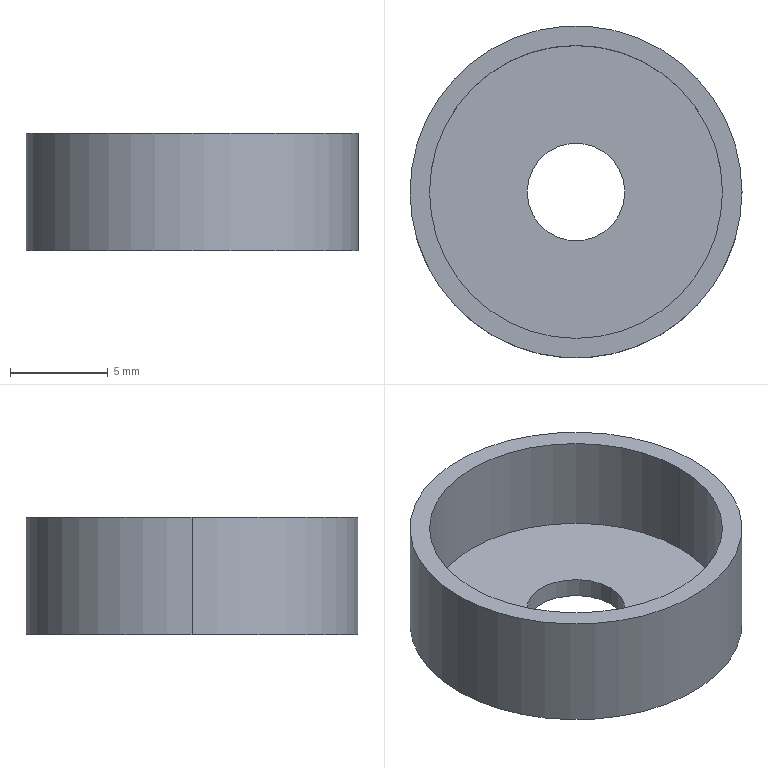Part | SolidWorks | features Extrusion 1, ICE 1 | 1 solid | 9 faces | box 17 x 17 x 6 mm | volume 458.673 mm3 | cylinder 6 | plane 3 | commonest cylinder face diameters 5 x2 15 x2 17 x2
STEP:
#1=CARTESIAN_POINT('',(-7.5,0.,1.));
#2=VERTEX_POINT('',#1);
#3=CARTESIAN_POINT('',(7.5,0.,1.));
#4=VERTEX_POINT('',#3);
#5=CARTESIAN_POINT('',(0.,0.,1.));
#6=DIRECTION('',(0.,0.,1.));
#7=DIRECTION('',(1.,0.,0.));
#8=AXIS2_PLACEMENT_3D('',#5,#6,#7);
#9=CIRCLE('',#8,7.5);
#10=EDGE_CURVE('',#2,#4,#9,.T.);
#11=ORIENTED_EDGE('',*,*,#10,.F.);
#12=CARTESIAN_POINT('',(-7.5,0.,6.));
#13=VERTEX_POINT('',#12);
#14=CARTESIAN_POINT('',(-7.5,0.,1.));
#15=DIRECTION('',(0.,0.,1.));
#16=VECTOR('',#15,1000.);
#17=LINE('',#14,#16);
#18=EDGE_CURVE('',#2,#13,#17,.T.);
#19=ORIENTED_EDGE('',*,*,#18,.T.);
#20=CARTESIAN_POINT('',(7.5,0.,6.));
#21=VERTEX_POINT('',#20);
#22=CARTESIAN_POINT('',(0.,0.,6.));
#23=DIRECTION('',(0.,0.,1.));
#24=DIRECTION('',(1.,0.,0.));
#25=AXIS2_PLACEMENT_3D('',#22,#23,#24);
#26=CIRCLE('',#25,7.5);
#27=EDGE_CURVE('',#13,#21,#26,.T.);
#28=ORIENTED_EDGE('',*,*,#27,.T.);
#29=CARTESIAN_POINT('',(7.5,0.,1.));
#30=DIRECTION('',(0.,0.,1.));
#31=VECTOR('',#30,1000.);
#32=LINE('',#29,#31);
#33=EDGE_CURVE('',#4,#21,#32,.T.);
#34=ORIENTED_EDGE('',*,*,#33,.F.);
#35=EDGE_LOOP('',(#11,#19,#28,#34));
#36=FACE_OUTER_BOUND('',#35,.T.);
#37=CARTESIAN_POINT('',(0.,0.,1.));
#38=DIRECTION('',(0.,0.,1.));
#39=DIRECTION('',(1.,0.,0.));
#40=AXIS2_PLACEMENT_3D('',#37,#38,#39);
#41=CYLINDRICAL_SURFACE('',#40,7.5);
#42=ADVANCED_FACE('',(#36),#41,.F.);
#43=CARTESIAN_POINT('',(8.5,0.,6.));
#44=VERTEX_POINT('',#43);
#45=CARTESIAN_POINT('',(-8.5,0.,6.));
#46=VERTEX_POINT('',#45);
#47=CARTESIAN_POINT('',(0.,0.,6.));
#48=DIRECTION('',(0.,0.,1.));
#49=DIRECTION('',(1.,0.,0.));
#50=AXIS2_PLACEMENT_3D('',#47,#48,#49);
#51=CIRCLE('',#50,8.5);
#52=EDGE_CURVE('',#44,#46,#51,.T.);
#53=ORIENTED_EDGE('',*,*,#52,.F.);
#54=CARTESIAN_POINT('',(8.5,0.,0.));
#55=VERTEX_POINT('',#54);
#56=CARTESIAN_POINT('',(8.5,0.,6.));
#57=DIRECTION('',(0.,0.,-1.));
#58=VECTOR('',#57,1000.);
#59=LINE('',#56,#58);
#60=EDGE_CURVE('',#44,#55,#59,.T.);
#61=ORIENTED_EDGE('',*,*,#60,.T.);
#62=CARTESIAN_POINT('',(-8.5,0.,0.));
#63=VERTEX_POINT('',#62);
#64=CARTESIAN_POINT('',(0.,0.,0.));
#65=DIRECTION('',(0.,0.,1.));
#66=DIRECTION('',(1.,0.,0.));
#67=AXIS2_PLACEMENT_3D('',#64,#65,#66);
#68=CIRCLE('',#67,8.5);
#69=EDGE_CURVE('',#55,#63,#68,.T.);
#70=ORIENTED_EDGE('',*,*,#69,.T.);
#71=CARTESIAN_POINT('',(-8.5,0.,6.));
#72=DIRECTION('',(0.,0.,-1.));
#73=VECTOR('',#72,1000.);
#74=LINE('',#71,#73);
#75=EDGE_CURVE('',#46,#63,#74,.T.);
#76=ORIENTED_EDGE('',*,*,#75,.F.);
#77=EDGE_LOOP('',(#53,#61,#70,#76));
#78=FACE_OUTER_BOUND('',#77,.T.);
#79=CARTESIAN_POINT('',(0.,0.,6.));
#80=DIRECTION('',(0.,0.,-1.));
#81=DIRECTION('',(-1.,0.,0.));
#82=AXIS2_PLACEMENT_3D('',#79,#80,#81);
#83=CYLINDRICAL_SURFACE('',#82,8.5);
#84=ADVANCED_FACE('',(#78),#83,.T.);
#85=CARTESIAN_POINT('',(-2.5,0.,1.));
#86=VERTEX_POINT('',#85);
#87=CARTESIAN_POINT('',(2.5,0.,1.));
#88=VERTEX_POINT('',#87);
#89=CARTESIAN_POINT('',(0.,0.,1.));
#90=DIRECTION('',(0.,0.,1.));
#91=DIRECTION('',(1.,0.,0.));
#92=AXIS2_PLACEMENT_3D('',#89,#90,#91);
#93=CIRCLE('',#92,2.5);
#94=EDGE_CURVE('',#86,#88,#93,.T.);
#95=ORIENTED_EDGE('',*,*,#94,.T.);
#96=CARTESIAN_POINT('',(2.5,0.,0.));
#97=VERTEX_POINT('',#96);
#98=CARTESIAN_POINT('',(2.5,0.,6.));
#99=DIRECTION('',(0.,0.,-1.));
#100=VECTOR('',#99,1000.);
#101=LINE('',#98,#100);
#102=EDGE_CURVE('',#88,#97,#101,.T.);
#103=ORIENTED_EDGE('',*,*,#102,.T.);
#104=CARTESIAN_POINT('',(-2.5,0.,0.));
#105=VERTEX_POINT('',#104);
#106=CARTESIAN_POINT('',(0.,0.,0.));
#107=DIRECTION('',(0.,0.,1.));
#108=DIRECTION('',(1.,0.,0.));
#109=AXIS2_PLACEMENT_3D('',#106,#107,#108);
#110=CIRCLE('',#109,2.5);
#111=EDGE_CURVE('',#105,#97,#110,.T.);
#112=ORIENTED_EDGE('',*,*,#111,.F.);
#113=CARTESIAN_POINT('',(-2.5,0.,6.));
#114=DIRECTION('',(0.,0.,-1.));
#115=VECTOR('',#114,1000.);
#116=LINE('',#113,#115);
#117=EDGE_CURVE('',#86,#105,#116,.T.);
#118=ORIENTED_EDGE('',*,*,#117,.F.);
#119=EDGE_LOOP('',(#95,#103,#112,#118));
#120=FACE_OUTER_BOUND('',#119,.T.);
#121=CARTESIAN_POINT('',(0.,0.,6.));
#122=DIRECTION('',(0.,0.,-1.));
#123=DIRECTION('',(-1.,0.,0.));
#124=AXIS2_PLACEMENT_3D('',#121,#122,#123);
#125=CYLINDRICAL_SURFACE('',#124,2.5);
#126=ADVANCED_FACE('',(#120),#125,.F.);
#127=ORIENTED_EDGE('',*,*,#102,.F.);
#128=CARTESIAN_POINT('',(0.,0.,1.));
#129=DIRECTION('',(0.,0.,1.));
#130=DIRECTION('',(1.,0.,0.));
#131=AXIS2_PLACEMENT_3D('',#128,#129,#130);
#132=CIRCLE('',#131,2.5);
#133=EDGE_CURVE('',#88,#86,#132,.T.);
#134=ORIENTED_EDGE('',*,*,#133,.T.);
#135=ORIENTED_EDGE('',*,*,#117,.T.);
#136=CARTESIAN_POINT('',(0.,0.,0.));
#137=DIRECTION('',(0.,0.,1.));
#138=DIRECTION('',(1.,0.,0.));
#139=AXIS2_PLACEMENT_3D('',#136,#137,#138);
#140=CIRCLE('',#139,2.5);
#141=EDGE_CURVE('',#97,#105,#140,.T.);
#142=ORIENTED_EDGE('',*,*,#141,.F.);
#143=EDGE_LOOP('',(#127,#134,#135,#142));
#144=FACE_OUTER_BOUND('',#143,.T.);
#145=CARTESIAN_POINT('',(0.,0.,6.));
#146=DIRECTION('',(0.,0.,-1.));
#147=DIRECTION('',(-1.,0.,0.));
#148=AXIS2_PLACEMENT_3D('',#145,#146,#147);
#149=CYLINDRICAL_SURFACE('',#148,2.5);
#150=ADVANCED_FACE('',(#144),#149,.F.);
#151=CARTESIAN_POINT('',(0.,0.,6.));
#152=DIRECTION('',(0.,0.,1.));
#153=DIRECTION('',(1.,0.,0.));
#154=AXIS2_PLACEMENT_3D('',#151,#152,#153);
#155=CIRCLE('',#154,7.5);
#156=EDGE_CURVE('',#21,#13,#155,.T.);
#157=ORIENTED_EDGE('',*,*,#156,.F.);
#158=ORIENTED_EDGE('',*,*,#27,.F.);
#159=EDGE_LOOP('',(#157,#158));
#160=FACE_BOUND('',#159,.T.);
#161=CARTESIAN_POINT('',(0.,0.,6.));
#162=DIRECTION('',(0.,0.,1.));
#163=DIRECTION('',(1.,0.,0.));
#164=AXIS2_PLACEMENT_3D('',#161,#162,#163);
#165=CIRCLE('',#164,8.5);
#166=EDGE_CURVE('',#46,#44,#165,.T.);
#167=ORIENTED_EDGE('',*,*,#166,.T.);
#168=ORIENTED_EDGE('',*,*,#52,.T.);
#169=EDGE_LOOP('',(#167,#168));
#170=FACE_OUTER_BOUND('',#169,.T.);
#171=CARTESIAN_POINT('',(0.,0.,6.));
#172=DIRECTION('',(0.,0.,1.));
#173=DIRECTION('',(1.,0.,0.));
#174=AXIS2_PLACEMENT_3D('',#171,#172,#173);
#175=PLANE('',#174);
#176=ADVANCED_FACE('',(#160,#170),#175,.T.);
#177=CARTESIAN_POINT('',(0.,0.,0.));
#178=DIRECTION('',(0.,0.,1.));
#179=DIRECTION('',(1.,0.,0.));
#180=AXIS2_PLACEMENT_3D('',#177,#178,#179);
#181=CIRCLE('',#180,8.5);
#182=EDGE_CURVE('',#63,#55,#181,.T.);
#183=ORIENTED_EDGE('',*,*,#182,.F.);
#184=ORIENTED_EDGE('',*,*,#69,.F.);
#185=EDGE_LOOP('',(#183,#184));
#186=FACE_OUTER_BOUND('',#185,.T.);
#187=ORIENTED_EDGE('',*,*,#111,.T.);
#188=ORIENTED_EDGE('',*,*,#141,.T.);
#189=EDGE_LOOP('',(#187,#188));
#190=FACE_BOUND('',#189,.T.);
#191=CARTESIAN_POINT('',(0.,0.,0.));
#192=DIRECTION('',(0.,0.,1.));
#193=DIRECTION('',(1.,0.,0.));
#194=AXIS2_PLACEMENT_3D('',#191,#192,#193);
#195=PLANE('',#194);
#196=ADVANCED_FACE('',(#186,#190),#195,.F.);
#197=ORIENTED_EDGE('',*,*,#60,.F.);
#198=ORIENTED_EDGE('',*,*,#166,.F.);
#199=ORIENTED_EDGE('',*,*,#75,.T.);
#200=ORIENTED_EDGE('',*,*,#182,.T.);
#201=EDGE_LOOP('',(#197,#198,#199,#200));
#202=FACE_OUTER_BOUND('',#201,.T.);
#203=CARTESIAN_POINT('',(0.,0.,6.));
#204=DIRECTION('',(0.,0.,-1.));
#205=DIRECTION('',(-1.,0.,0.));
#206=AXIS2_PLACEMENT_3D('',#203,#204,#205);
#207=CYLINDRICAL_SURFACE('',#206,8.5);
#208=ADVANCED_FACE('',(#202),#207,.T.);
#209=ORIENTED_EDGE('',*,*,#18,.F.);
#210=CARTESIAN_POINT('',(0.,0.,1.));
#211=DIRECTION('',(0.,0.,1.));
#212=DIRECTION('',(1.,0.,0.));
#213=AXIS2_PLACEMENT_3D('',#210,#211,#212);
#214=CIRCLE('',#213,7.5);
#215=EDGE_CURVE('',#4,#2,#214,.T.);
#216=ORIENTED_EDGE('',*,*,#215,.F.);
#217=ORIENTED_EDGE('',*,*,#33,.T.);
#218=ORIENTED_EDGE('',*,*,#156,.T.);
#219=EDGE_LOOP('',(#209,#216,#217,#218));
#220=FACE_OUTER_BOUND('',#219,.T.);
#221=CARTESIAN_POINT('',(0.,0.,1.));
#222=DIRECTION('',(0.,0.,1.));
#223=DIRECTION('',(1.,0.,0.));
#224=AXIS2_PLACEMENT_3D('',#221,#222,#223);
#225=CYLINDRICAL_SURFACE('',#224,7.5);
#226=ADVANCED_FACE('',(#220),#225,.F.);
#227=ORIENTED_EDGE('',*,*,#94,.F.);
#228=ORIENTED_EDGE('',*,*,#133,.F.);
#229=EDGE_LOOP('',(#227,#228));
#230=FACE_BOUND('',#229,.T.);
#231=ORIENTED_EDGE('',*,*,#215,.T.);
#232=ORIENTED_EDGE('',*,*,#10,.T.);
#233=EDGE_LOOP('',(#231,#232));
#234=FACE_OUTER_BOUND('',#233,.T.);
#235=CARTESIAN_POINT('',(0.,0.,1.));
#236=DIRECTION('',(0.,0.,1.));
#237=DIRECTION('',(1.,0.,0.));
#238=AXIS2_PLACEMENT_3D('',#235,#236,#237);
#239=PLANE('',#238);
#240=ADVANCED_FACE('',(#230,#234),#239,.T.);
#241=CLOSED_SHELL('',(#42,#84,#126,#150,#176,#196,#208,#226,#240));
#242=MANIFOLD_SOLID_BREP('',#241);
#243=CARTESIAN_POINT('',(0.,0.,0.));
#244=DIRECTION('',(0.,0.,1.));
#245=DIRECTION('',(1.,0.,0.));
#246=AXIS2_PLACEMENT_3D('',#243,#244,#245);
#247=(LENGTH_UNIT()NAMED_UNIT(*)SI_UNIT(.MILLI.,.METRE.));
#248=UNCERTAINTY_MEASURE_WITH_UNIT(LENGTH_MEASURE(0.00001),#247,'','');
#249=(NAMED_UNIT(*)PLANE_ANGLE_UNIT()SI_UNIT($,.RADIAN.));
#250=(NAMED_UNIT(*)SI_UNIT($,.STERADIAN.)SOLID_ANGLE_UNIT());
#251=(GEOMETRIC_REPRESENTATION_CONTEXT(3)GLOBAL_UNCERTAINTY_ASSIGNED_CONTEXT((#248))GLOBAL_UNIT_ASSIGNED_CONTEXT((#247,#249,#250))REPRESENTATION_CONTEXT('',''));
#252=ADVANCED_BREP_SHAPE_REPRESENTATION('',(#242,#246),#251);